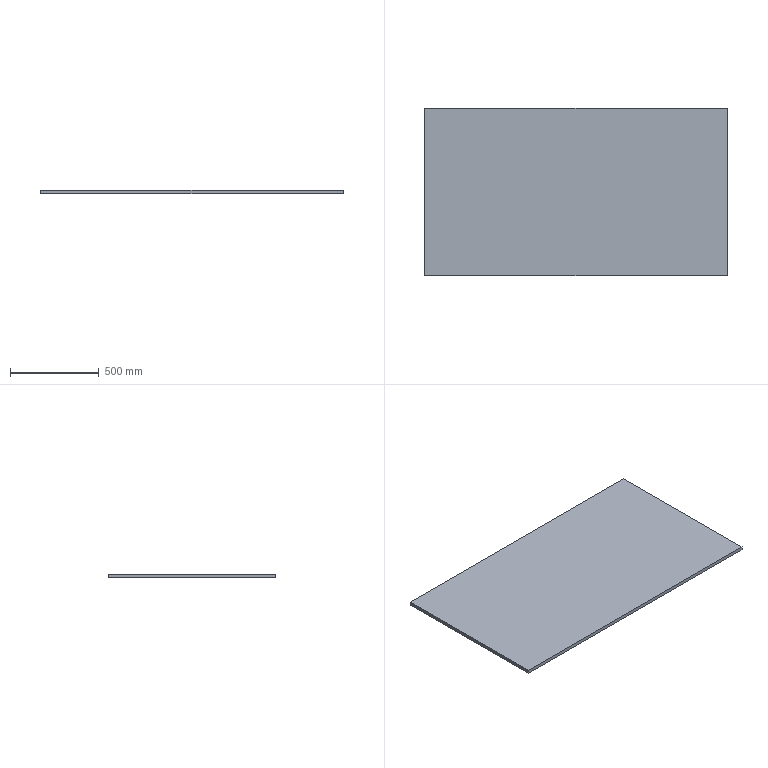Part | STEP file | 001-001-Main load plate | 1 solid | 6 faces | box 1700 x 940 x 20 mm | volume 31960000 mm3 | plane 6
STEP:
#1=CARTESIAN_POINT('',(0.,0.,0.));
#2=DIRECTION('',(0.,0.,1.));
#3=DIRECTION('',(1.,0.,0.));
#4=AXIS2_PLACEMENT_3D('',#1,#2,#3);
#5=CARTESIAN_POINT('',(-850.,470.,0.));
#6=VERTEX_POINT('',#5);
#7=CARTESIAN_POINT('',(-850.,-470.,0.));
#8=VERTEX_POINT('',#7);
#9=CARTESIAN_POINT('',(-850.,470.,0.));
#10=DIRECTION('',(0.,-1.,0.));
#11=VECTOR('',#10,1.);
#12=LINE('',#9,#11);
#13=CARTESIAN_POINT('',(-850.,470.,20.));
#14=DIRECTION('',(1.,0.,0.));
#15=DIRECTION('',(0.,1.,0.));
#16=AXIS2_PLACEMENT_3D('',#13,#14,#15);
#17=PLANE('',#16);
#18=CARTESIAN_POINT('',(0.,-20.));
#19=DIRECTION('',(-1.,0.));
#20=VECTOR('',#19,1.);
#21=LINE('',#18,#20);
#22=(GEOMETRIC_REPRESENTATION_CONTEXT(2)PARAMETRIC_REPRESENTATION_CONTEXT()REPRESENTATION_CONTEXT('',''));
#23=DEFINITIONAL_REPRESENTATION('',(#21),#22);
#24=PCURVE('',#17,#23);
#25=CARTESIAN_POINT('',(0.,0.,0.));
#26=DIRECTION('',(0.,0.,1.));
#27=DIRECTION('',(1.,0.,0.));
#28=AXIS2_PLACEMENT_3D('',#25,#26,#27);
#29=PLANE('',#28);
#30=CARTESIAN_POINT('',(-850.,470.));
#31=DIRECTION('',(0.,-1.));
#32=VECTOR('',#31,1.);
#33=LINE('',#30,#32);
#34=(GEOMETRIC_REPRESENTATION_CONTEXT(2)PARAMETRIC_REPRESENTATION_CONTEXT()REPRESENTATION_CONTEXT('',''));
#35=DEFINITIONAL_REPRESENTATION('',(#33),#34);
#36=PCURVE('',#29,#35);
#37=SURFACE_CURVE('',#12,(#24,#36),.PCURVE_S1.);
#38=EDGE_CURVE('',#6,#8,#37,.T.);
#39=ORIENTED_EDGE('',*,*,#38,.T.);
#40=CARTESIAN_POINT('',(-850.,-470.,20.));
#41=VERTEX_POINT('',#40);
#42=CARTESIAN_POINT('',(-850.,-470.,20.));
#43=DIRECTION('',(0.,0.,-1.));
#44=VECTOR('',#43,1.);
#45=LINE('',#42,#44);
#46=CARTESIAN_POINT('',(-940.,0.));
#47=DIRECTION('',(0.,-1.));
#48=VECTOR('',#47,1.);
#49=LINE('',#46,#48);
#50=(GEOMETRIC_REPRESENTATION_CONTEXT(2)PARAMETRIC_REPRESENTATION_CONTEXT()REPRESENTATION_CONTEXT('',''));
#51=DEFINITIONAL_REPRESENTATION('',(#49),#50);
#52=PCURVE('',#17,#51);
#53=CARTESIAN_POINT('',(-850.,-470.,20.));
#54=DIRECTION('',(0.,1.,0.));
#55=DIRECTION('',(0.,0.,1.));
#56=AXIS2_PLACEMENT_3D('',#53,#54,#55);
#57=PLANE('',#56);
#58=CARTESIAN_POINT('',(0.,0.));
#59=DIRECTION('',(-1.,0.));
#60=VECTOR('',#59,1.);
#61=LINE('',#58,#60);
#62=(GEOMETRIC_REPRESENTATION_CONTEXT(2)PARAMETRIC_REPRESENTATION_CONTEXT()REPRESENTATION_CONTEXT('',''));
#63=DEFINITIONAL_REPRESENTATION('',(#61),#62);
#64=PCURVE('',#57,#63);
#65=SURFACE_CURVE('',#45,(#52,#64),.PCURVE_S1.);
#66=EDGE_CURVE('',#41,#8,#65,.T.);
#67=ORIENTED_EDGE('',*,*,#66,.F.);
#68=CARTESIAN_POINT('',(-850.,470.,20.));
#69=VERTEX_POINT('',#68);
#70=CARTESIAN_POINT('',(-850.,470.,20.));
#71=DIRECTION('',(0.,-1.,0.));
#72=VECTOR('',#71,1.);
#73=LINE('',#70,#72);
#74=CARTESIAN_POINT('',(0.,0.));
#75=DIRECTION('',(-1.,0.));
#76=VECTOR('',#75,1.);
#77=LINE('',#74,#76);
#78=(GEOMETRIC_REPRESENTATION_CONTEXT(2)PARAMETRIC_REPRESENTATION_CONTEXT()REPRESENTATION_CONTEXT('',''));
#79=DEFINITIONAL_REPRESENTATION('',(#77),#78);
#80=PCURVE('',#17,#79);
#81=CARTESIAN_POINT('',(0.,0.,20.));
#82=DIRECTION('',(0.,0.,1.));
#83=DIRECTION('',(1.,0.,0.));
#84=AXIS2_PLACEMENT_3D('',#81,#82,#83);
#85=PLANE('',#84);
#86=CARTESIAN_POINT('',(-850.,470.));
#87=DIRECTION('',(0.,-1.));
#88=VECTOR('',#87,1.);
#89=LINE('',#86,#88);
#90=(GEOMETRIC_REPRESENTATION_CONTEXT(2)PARAMETRIC_REPRESENTATION_CONTEXT()REPRESENTATION_CONTEXT('',''));
#91=DEFINITIONAL_REPRESENTATION('',(#89),#90);
#92=PCURVE('',#85,#91);
#93=SURFACE_CURVE('',#73,(#80,#92),.PCURVE_S1.);
#94=EDGE_CURVE('',#69,#41,#93,.T.);
#95=ORIENTED_EDGE('',*,*,#94,.F.);
#96=CARTESIAN_POINT('',(-850.,470.,20.));
#97=DIRECTION('',(0.,0.,-1.));
#98=VECTOR('',#97,1.);
#99=LINE('',#96,#98);
#100=CARTESIAN_POINT('',(0.,0.));
#101=DIRECTION('',(0.,-1.));
#102=VECTOR('',#101,1.);
#103=LINE('',#100,#102);
#104=(GEOMETRIC_REPRESENTATION_CONTEXT(2)PARAMETRIC_REPRESENTATION_CONTEXT()REPRESENTATION_CONTEXT('',''));
#105=DEFINITIONAL_REPRESENTATION('',(#103),#104);
#106=PCURVE('',#17,#105);
#107=CARTESIAN_POINT('',(-850.,470.,20.));
#108=DIRECTION('',(0.,-1.,0.));
#109=DIRECTION('',(0.,0.,-1.));
#110=AXIS2_PLACEMENT_3D('',#107,#108,#109);
#111=PLANE('',#110);
#112=CARTESIAN_POINT('',(0.,0.));
#113=DIRECTION('',(1.,0.));
#114=VECTOR('',#113,1.);
#115=LINE('',#112,#114);
#116=(GEOMETRIC_REPRESENTATION_CONTEXT(2)PARAMETRIC_REPRESENTATION_CONTEXT()REPRESENTATION_CONTEXT('',''));
#117=DEFINITIONAL_REPRESENTATION('',(#115),#116);
#118=PCURVE('',#111,#117);
#119=SURFACE_CURVE('',#99,(#106,#118),.PCURVE_S1.);
#120=EDGE_CURVE('',#69,#6,#119,.T.);
#121=ORIENTED_EDGE('',*,*,#120,.T.);
#122=EDGE_LOOP('',(#39,#67,#95,#121));
#123=FACE_BOUND('',#122,.T.);
#124=ADVANCED_FACE('',(#123),#17,.F.);
#125=CARTESIAN_POINT('',(850.,-470.,0.));
#126=VERTEX_POINT('',#125);
#127=CARTESIAN_POINT('',(-850.,-470.,0.));
#128=DIRECTION('',(1.,0.,0.));
#129=VECTOR('',#128,1.);
#130=LINE('',#127,#129);
#131=CARTESIAN_POINT('',(-20.,0.));
#132=DIRECTION('',(0.,1.));
#133=VECTOR('',#132,1.);
#134=LINE('',#131,#133);
#135=(GEOMETRIC_REPRESENTATION_CONTEXT(2)PARAMETRIC_REPRESENTATION_CONTEXT()REPRESENTATION_CONTEXT('',''));
#136=DEFINITIONAL_REPRESENTATION('',(#134),#135);
#137=PCURVE('',#57,#136);
#138=CARTESIAN_POINT('',(-850.,-470.));
#139=DIRECTION('',(1.,0.));
#140=VECTOR('',#139,1.);
#141=LINE('',#138,#140);
#142=(GEOMETRIC_REPRESENTATION_CONTEXT(2)PARAMETRIC_REPRESENTATION_CONTEXT()REPRESENTATION_CONTEXT('',''));
#143=DEFINITIONAL_REPRESENTATION('',(#141),#142);
#144=PCURVE('',#29,#143);
#145=SURFACE_CURVE('',#130,(#137,#144),.PCURVE_S1.);
#146=EDGE_CURVE('',#8,#126,#145,.T.);
#147=ORIENTED_EDGE('',*,*,#146,.T.);
#148=CARTESIAN_POINT('',(850.,-470.,20.));
#149=VERTEX_POINT('',#148);
#150=CARTESIAN_POINT('',(850.,-470.,20.));
#151=DIRECTION('',(0.,0.,-1.));
#152=VECTOR('',#151,1.);
#153=LINE('',#150,#152);
#154=CARTESIAN_POINT('',(0.,1700.));
#155=DIRECTION('',(-1.,0.));
#156=VECTOR('',#155,1.);
#157=LINE('',#154,#156);
#158=(GEOMETRIC_REPRESENTATION_CONTEXT(2)PARAMETRIC_REPRESENTATION_CONTEXT()REPRESENTATION_CONTEXT('',''));
#159=DEFINITIONAL_REPRESENTATION('',(#157),#158);
#160=PCURVE('',#57,#159);
#161=CARTESIAN_POINT('',(850.,470.,20.));
#162=DIRECTION('',(-1.,0.,0.));
#163=DIRECTION('',(0.,-1.,0.));
#164=AXIS2_PLACEMENT_3D('',#161,#162,#163);
#165=PLANE('',#164);
#166=CARTESIAN_POINT('',(940.,0.));
#167=DIRECTION('',(0.,-1.));
#168=VECTOR('',#167,1.);
#169=LINE('',#166,#168);
#170=(GEOMETRIC_REPRESENTATION_CONTEXT(2)PARAMETRIC_REPRESENTATION_CONTEXT()REPRESENTATION_CONTEXT('',''));
#171=DEFINITIONAL_REPRESENTATION('',(#169),#170);
#172=PCURVE('',#165,#171);
#173=SURFACE_CURVE('',#153,(#160,#172),.PCURVE_S1.);
#174=EDGE_CURVE('',#149,#126,#173,.T.);
#175=ORIENTED_EDGE('',*,*,#174,.F.);
#176=CARTESIAN_POINT('',(-850.,-470.,20.));
#177=DIRECTION('',(1.,0.,0.));
#178=VECTOR('',#177,1.);
#179=LINE('',#176,#178);
#180=CARTESIAN_POINT('',(0.,0.));
#181=DIRECTION('',(0.,1.));
#182=VECTOR('',#181,1.);
#183=LINE('',#180,#182);
#184=(GEOMETRIC_REPRESENTATION_CONTEXT(2)PARAMETRIC_REPRESENTATION_CONTEXT()REPRESENTATION_CONTEXT('',''));
#185=DEFINITIONAL_REPRESENTATION('',(#183),#184);
#186=PCURVE('',#57,#185);
#187=CARTESIAN_POINT('',(-850.,-470.));
#188=DIRECTION('',(1.,0.));
#189=VECTOR('',#188,1.);
#190=LINE('',#187,#189);
#191=(GEOMETRIC_REPRESENTATION_CONTEXT(2)PARAMETRIC_REPRESENTATION_CONTEXT()REPRESENTATION_CONTEXT('',''));
#192=DEFINITIONAL_REPRESENTATION('',(#190),#191);
#193=PCURVE('',#85,#192);
#194=SURFACE_CURVE('',#179,(#186,#193),.PCURVE_S1.);
#195=EDGE_CURVE('',#41,#149,#194,.T.);
#196=ORIENTED_EDGE('',*,*,#195,.F.);
#197=ORIENTED_EDGE('',*,*,#66,.T.);
#198=EDGE_LOOP('',(#147,#175,#196,#197));
#199=FACE_BOUND('',#198,.T.);
#200=ADVANCED_FACE('',(#199),#57,.F.);
#201=CARTESIAN_POINT('',(850.,470.,0.));
#202=VERTEX_POINT('',#201);
#203=CARTESIAN_POINT('',(850.,470.,0.));
#204=DIRECTION('',(0.,1.,0.));
#205=VECTOR('',#204,1.);
#206=LINE('',#203,#205);
#207=CARTESIAN_POINT('',(0.,-20.));
#208=DIRECTION('',(-1.,0.));
#209=VECTOR('',#208,1.);
#210=LINE('',#207,#209);
#211=(GEOMETRIC_REPRESENTATION_CONTEXT(2)PARAMETRIC_REPRESENTATION_CONTEXT()REPRESENTATION_CONTEXT('',''));
#212=DEFINITIONAL_REPRESENTATION('',(#210),#211);
#213=PCURVE('',#165,#212);
#214=CARTESIAN_POINT('',(850.,470.));
#215=DIRECTION('',(0.,1.));
#216=VECTOR('',#215,1.);
#217=LINE('',#214,#216);
#218=(GEOMETRIC_REPRESENTATION_CONTEXT(2)PARAMETRIC_REPRESENTATION_CONTEXT()REPRESENTATION_CONTEXT('',''));
#219=DEFINITIONAL_REPRESENTATION('',(#217),#218);
#220=PCURVE('',#29,#219);
#221=SURFACE_CURVE('',#206,(#213,#220),.PCURVE_S1.);
#222=EDGE_CURVE('',#126,#202,#221,.T.);
#223=ORIENTED_EDGE('',*,*,#222,.T.);
#224=CARTESIAN_POINT('',(850.,470.,20.));
#225=VERTEX_POINT('',#224);
#226=CARTESIAN_POINT('',(850.,470.,20.));
#227=DIRECTION('',(0.,0.,-1.));
#228=VECTOR('',#227,1.);
#229=LINE('',#226,#228);
#230=CARTESIAN_POINT('',(0.,0.));
#231=DIRECTION('',(0.,-1.));
#232=VECTOR('',#231,1.);
#233=LINE('',#230,#232);
#234=(GEOMETRIC_REPRESENTATION_CONTEXT(2)PARAMETRIC_REPRESENTATION_CONTEXT()REPRESENTATION_CONTEXT('',''));
#235=DEFINITIONAL_REPRESENTATION('',(#233),#234);
#236=PCURVE('',#165,#235);
#237=CARTESIAN_POINT('',(0.,1700.));
#238=DIRECTION('',(1.,0.));
#239=VECTOR('',#238,1.);
#240=LINE('',#237,#239);
#241=(GEOMETRIC_REPRESENTATION_CONTEXT(2)PARAMETRIC_REPRESENTATION_CONTEXT()REPRESENTATION_CONTEXT('',''));
#242=DEFINITIONAL_REPRESENTATION('',(#240),#241);
#243=PCURVE('',#111,#242);
#244=SURFACE_CURVE('',#229,(#236,#243),.PCURVE_S1.);
#245=EDGE_CURVE('',#225,#202,#244,.T.);
#246=ORIENTED_EDGE('',*,*,#245,.F.);
#247=CARTESIAN_POINT('',(850.,470.,20.));
#248=DIRECTION('',(0.,1.,0.));
#249=VECTOR('',#248,1.);
#250=LINE('',#247,#249);
#251=CARTESIAN_POINT('',(0.,0.));
#252=DIRECTION('',(-1.,0.));
#253=VECTOR('',#252,1.);
#254=LINE('',#251,#253);
#255=(GEOMETRIC_REPRESENTATION_CONTEXT(2)PARAMETRIC_REPRESENTATION_CONTEXT()REPRESENTATION_CONTEXT('',''));
#256=DEFINITIONAL_REPRESENTATION('',(#254),#255);
#257=PCURVE('',#165,#256);
#258=CARTESIAN_POINT('',(850.,470.));
#259=DIRECTION('',(0.,1.));
#260=VECTOR('',#259,1.);
#261=LINE('',#258,#260);
#262=(GEOMETRIC_REPRESENTATION_CONTEXT(2)PARAMETRIC_REPRESENTATION_CONTEXT()REPRESENTATION_CONTEXT('',''));
#263=DEFINITIONAL_REPRESENTATION('',(#261),#262);
#264=PCURVE('',#85,#263);
#265=SURFACE_CURVE('',#250,(#257,#264),.PCURVE_S1.);
#266=EDGE_CURVE('',#149,#225,#265,.T.);
#267=ORIENTED_EDGE('',*,*,#266,.F.);
#268=ORIENTED_EDGE('',*,*,#174,.T.);
#269=EDGE_LOOP('',(#223,#246,#267,#268));
#270=FACE_BOUND('',#269,.T.);
#271=ADVANCED_FACE('',(#270),#165,.F.);
#272=CARTESIAN_POINT('',(-850.,470.,0.));
#273=DIRECTION('',(-1.,0.,0.));
#274=VECTOR('',#273,1.);
#275=LINE('',#272,#274);
#276=CARTESIAN_POINT('',(20.,0.));
#277=DIRECTION('',(0.,-1.));
#278=VECTOR('',#277,1.);
#279=LINE('',#276,#278);
#280=(GEOMETRIC_REPRESENTATION_CONTEXT(2)PARAMETRIC_REPRESENTATION_CONTEXT()REPRESENTATION_CONTEXT('',''));
#281=DEFINITIONAL_REPRESENTATION('',(#279),#280);
#282=PCURVE('',#111,#281);
#283=CARTESIAN_POINT('',(-850.,470.));
#284=DIRECTION('',(-1.,0.));
#285=VECTOR('',#284,1.);
#286=LINE('',#283,#285);
#287=(GEOMETRIC_REPRESENTATION_CONTEXT(2)PARAMETRIC_REPRESENTATION_CONTEXT()REPRESENTATION_CONTEXT('',''));
#288=DEFINITIONAL_REPRESENTATION('',(#286),#287);
#289=PCURVE('',#29,#288);
#290=SURFACE_CURVE('',#275,(#282,#289),.PCURVE_S1.);
#291=EDGE_CURVE('',#202,#6,#290,.T.);
#292=ORIENTED_EDGE('',*,*,#291,.T.);
#293=ORIENTED_EDGE('',*,*,#120,.F.);
#294=CARTESIAN_POINT('',(-850.,470.,20.));
#295=DIRECTION('',(-1.,0.,0.));
#296=VECTOR('',#295,1.);
#297=LINE('',#294,#296);
#298=CARTESIAN_POINT('',(0.,0.));
#299=DIRECTION('',(0.,-1.));
#300=VECTOR('',#299,1.);
#301=LINE('',#298,#300);
#302=(GEOMETRIC_REPRESENTATION_CONTEXT(2)PARAMETRIC_REPRESENTATION_CONTEXT()REPRESENTATION_CONTEXT('',''));
#303=DEFINITIONAL_REPRESENTATION('',(#301),#302);
#304=PCURVE('',#111,#303);
#305=CARTESIAN_POINT('',(-850.,470.));
#306=DIRECTION('',(-1.,0.));
#307=VECTOR('',#306,1.);
#308=LINE('',#305,#307);
#309=(GEOMETRIC_REPRESENTATION_CONTEXT(2)PARAMETRIC_REPRESENTATION_CONTEXT()REPRESENTATION_CONTEXT('',''));
#310=DEFINITIONAL_REPRESENTATION('',(#308),#309);
#311=PCURVE('',#85,#310);
#312=SURFACE_CURVE('',#297,(#304,#311),.PCURVE_S1.);
#313=EDGE_CURVE('',#225,#69,#312,.T.);
#314=ORIENTED_EDGE('',*,*,#313,.F.);
#315=ORIENTED_EDGE('',*,*,#245,.T.);
#316=EDGE_LOOP('',(#292,#293,#314,#315));
#317=FACE_BOUND('',#316,.T.);
#318=ADVANCED_FACE('',(#317),#111,.F.);
#319=ORIENTED_EDGE('',*,*,#94,.T.);
#320=ORIENTED_EDGE('',*,*,#195,.T.);
#321=ORIENTED_EDGE('',*,*,#266,.T.);
#322=ORIENTED_EDGE('',*,*,#313,.T.);
#323=EDGE_LOOP('',(#319,#320,#321,#322));
#324=FACE_BOUND('',#323,.T.);
#325=ADVANCED_FACE('',(#324),#85,.T.);
#326=ORIENTED_EDGE('',*,*,#38,.F.);
#327=ORIENTED_EDGE('',*,*,#291,.F.);
#328=ORIENTED_EDGE('',*,*,#222,.F.);
#329=ORIENTED_EDGE('',*,*,#146,.F.);
#330=EDGE_LOOP('',(#326,#327,#328,#329));
#331=FACE_BOUND('',#330,.T.);
#332=ADVANCED_FACE('',(#331),#29,.F.);
#333=CLOSED_SHELL('',(#124,#200,#271,#318,#325,#332));
#334=MANIFOLD_SOLID_BREP('',#333);
#335=(LENGTH_UNIT()NAMED_UNIT(*)SI_UNIT(.MILLI.,.METRE.));
#336=UNCERTAINTY_MEASURE_WITH_UNIT(LENGTH_MEASURE(0.0000001),#335,'','');
#337=(NAMED_UNIT(*)PLANE_ANGLE_UNIT()SI_UNIT($,.RADIAN.));
#338=(NAMED_UNIT(*)SI_UNIT($,.STERADIAN.)SOLID_ANGLE_UNIT());
#339=(GEOMETRIC_REPRESENTATION_CONTEXT(3)GLOBAL_UNCERTAINTY_ASSIGNED_CONTEXT((#336))GLOBAL_UNIT_ASSIGNED_CONTEXT((#335,#337,#338))REPRESENTATION_CONTEXT('',''));
#340=ADVANCED_BREP_SHAPE_REPRESENTATION('',(#4,#334),#339);